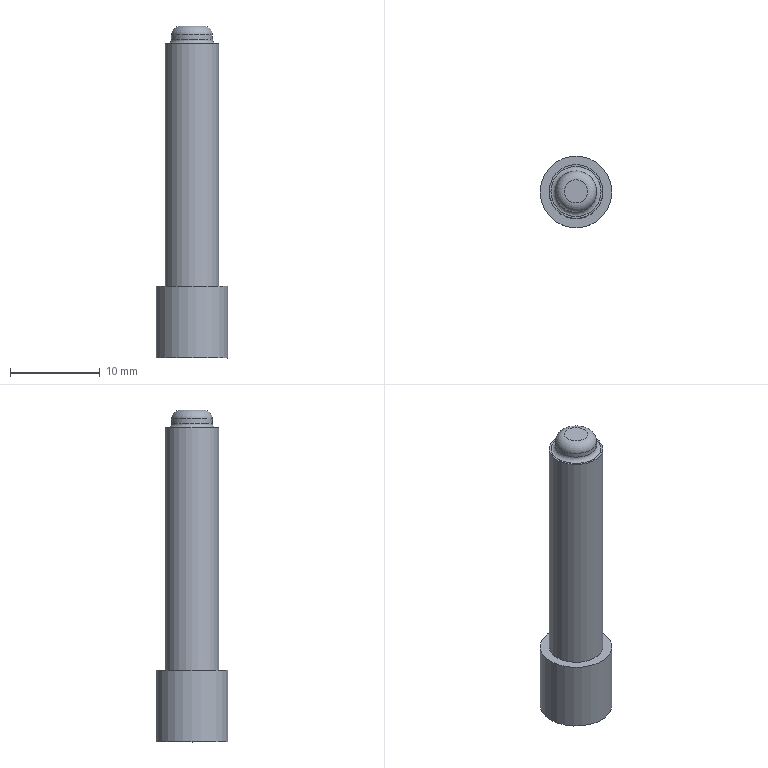Part | NX | features solid 2 | 1 solid | 9 faces | box 8 x 8 x 37 mm | volume 1197 mm3 | plane 4 | cylinder 3 | torus 2 | commonest cylinder face diameters 4.58 x1 6 x1 8 x1
STEP:
#1=CARTESIAN_POINT('',(4220.236,-877.122,858.716));
#2=VERTEX_POINT('',#1);
#3=CARTESIAN_POINT('',(4217.236,-877.122,858.716));
#4=DIRECTION('',(0.,0.,1.));
#5=DIRECTION('',(1.,0.,0.));
#6=AXIS2_PLACEMENT_3D('',#3,#4,#5);
#7=CIRCLE('',#6,3.);
#8=EDGE_CURVE('',#2,#2,#7,.T.);
#9=ORIENTED_EDGE('',*,*,#8,.F.);
#10=EDGE_LOOP('',(#9));
#11=FACE_BOUND('',#10,.T.);
#12=CARTESIAN_POINT('',(4214.236,-877.122,831.716));
#13=VERTEX_POINT('',#12);
#14=CARTESIAN_POINT('',(4217.236,-877.122,831.716));
#15=DIRECTION('',(0.,0.,-1.));
#16=DIRECTION('',(-1.,0.,0.));
#17=AXIS2_PLACEMENT_3D('',#14,#15,#16);
#18=CIRCLE('',#17,3.);
#19=EDGE_CURVE('',#13,#13,#18,.F.);
#20=ORIENTED_EDGE('',*,*,#19,.T.);
#21=EDGE_LOOP('',(#20));
#22=FACE_BOUND('',#21,.T.);
#23=CARTESIAN_POINT('',(4217.236,-877.122,823.716));
#24=DIRECTION('',(0.,0.,1.));
#25=DIRECTION('',(1.,0.,0.));
#26=AXIS2_PLACEMENT_3D('',#23,#24,#25);
#27=CYLINDRICAL_SURFACE('',#26,3.);
#28=ADVANCED_FACE('',(#11,#22),#27,.T.);
#29=CARTESIAN_POINT('',(4214.997,-877.601,859.716));
#30=VERTEX_POINT('',#29);
#31=CARTESIAN_POINT('',(4215.858,-879.254,859.716));
#32=CARTESIAN_POINT('',(4214.754,-877.652,859.716));
#33=CARTESIAN_POINT('',(4215.107,-875.742,859.716));
#34=CARTESIAN_POINT('',(4216.704,-874.641,859.716));
#35=CARTESIAN_POINT('',(4218.615,-874.991,859.716));
#36=CARTESIAN_POINT('',(4219.718,-876.591,859.716));
#37=CARTESIAN_POINT('',(4219.367,-878.499,859.716));
#38=CARTESIAN_POINT('',(4217.769,-879.603,859.716));
#39=CARTESIAN_POINT('',(4215.858,-879.254,859.716));
#40=CARTESIAN_POINT('',(4214.754,-877.652,859.716));
#41=CARTESIAN_POINT('',(4215.107,-875.742,859.716));
#42=B_SPLINE_CURVE_WITH_KNOTS('',3,(#31,#32,#33,#34,#35,#36,#37,#38,#39,#40,#41),.UNSPECIFIED.,.T.,.F.,(1,1,1,1,1,1,1,1,1,1,1,1,1,1,1),(-0.005369,-0.003579,-0.00179,0.,0.00179,0.003579,0.005369,0.007159,0.008948,0.01074,0.01253,0.01432,0.01611,0.0179,0.01969),.UNSPECIFIED.);
#43=EDGE_CURVE('',#30,#30,#42,.T.);
#44=ORIENTED_EDGE('',*,*,#43,.T.);
#45=EDGE_LOOP('',(#44));
#46=FACE_BOUND('',#45,.T.);
#47=CARTESIAN_POINT('',(4219.526,-877.122,859.216));
#48=VERTEX_POINT('',#47);
#49=CARTESIAN_POINT('',(4217.236,-877.122,859.216));
#50=DIRECTION('',(0.,0.,1.));
#51=DIRECTION('',(1.,0.,0.));
#52=AXIS2_PLACEMENT_3D('',#49,#50,#51);
#53=CIRCLE('',#52,2.29);
#54=EDGE_CURVE('',#48,#48,#53,.F.);
#55=ORIENTED_EDGE('',*,*,#54,.F.);
#56=EDGE_LOOP('',(#55));
#57=FACE_BOUND('',#56,.T.);
#58=CARTESIAN_POINT('',(4217.236,-877.122,860.716));
#59=DIRECTION('',(0.,0.,-1.));
#60=DIRECTION('',(-1.,0.,0.));
#61=AXIS2_PLACEMENT_3D('',#58,#59,#60);
#62=CYLINDRICAL_SURFACE('',#61,2.29);
#63=ADVANCED_FACE('',(#46,#57),#62,.T.);
#64=CARTESIAN_POINT('',(4215.946,-877.122,860.716));
#65=VERTEX_POINT('',#64);
#66=CARTESIAN_POINT('',(4217.236,-877.122,860.716));
#67=DIRECTION('',(0.,0.,-1.));
#68=DIRECTION('',(-1.,0.,0.));
#69=AXIS2_PLACEMENT_3D('',#66,#67,#68);
#70=CIRCLE('',#69,1.29);
#71=EDGE_CURVE('',#65,#65,#70,.F.);
#72=ORIENTED_EDGE('',*,*,#71,.T.);
#73=EDGE_LOOP('',(#72));
#74=FACE_BOUND('',#73,.T.);
#75=CARTESIAN_POINT('',(4217.236,-877.122,860.716));
#76=DIRECTION('',(0.,0.,-1.));
#77=DIRECTION('',(-1.,0.,0.));
#78=AXIS2_PLACEMENT_3D('',#75,#76,#77);
#79=PLANE('',#78);
#80=ADVANCED_FACE('',(#74),#79,.F.);
#81=CARTESIAN_POINT('',(4220.026,-877.122,858.716));
#82=VERTEX_POINT('',#81);
#83=CARTESIAN_POINT('',(4217.236,-877.122,858.716));
#84=DIRECTION('',(0.,0.,1.));
#85=DIRECTION('',(1.,0.,0.));
#86=AXIS2_PLACEMENT_3D('',#83,#84,#85);
#87=CIRCLE('',#86,2.79);
#88=EDGE_CURVE('',#82,#82,#87,.F.);
#89=ORIENTED_EDGE('',*,*,#88,.F.);
#90=EDGE_LOOP('',(#89));
#91=FACE_BOUND('',#90,.T.);
#92=ORIENTED_EDGE('',*,*,#54,.T.);
#93=EDGE_LOOP('',(#92));
#94=FACE_BOUND('',#93,.T.);
#95=CARTESIAN_POINT('',(4217.236,-877.122,859.216));
#96=DIRECTION('',(0.,0.,1.));
#97=DIRECTION('',(1.,0.,0.));
#98=AXIS2_PLACEMENT_3D('',#95,#96,#97);
#99=TOROIDAL_SURFACE('',#98,2.79,0.5);
#100=ADVANCED_FACE('',(#91,#94),#99,.F.);
#101=ORIENTED_EDGE('',*,*,#88,.T.);
#102=EDGE_LOOP('',(#101));
#103=FACE_BOUND('',#102,.T.);
#104=ORIENTED_EDGE('',*,*,#8,.T.);
#105=EDGE_LOOP('',(#104));
#106=FACE_BOUND('',#105,.T.);
#107=CARTESIAN_POINT('',(4217.236,-839.122,858.716));
#108=DIRECTION('',(0.,0.,1.));
#109=DIRECTION('',(1.,0.,0.));
#110=AXIS2_PLACEMENT_3D('',#107,#108,#109);
#111=PLANE('',#110);
#112=ADVANCED_FACE('',(#103,#106),#111,.T.);
#113=ORIENTED_EDGE('',*,*,#71,.F.);
#114=EDGE_LOOP('',(#113));
#115=FACE_BOUND('',#114,.T.);
#116=ORIENTED_EDGE('',*,*,#43,.F.);
#117=EDGE_LOOP('',(#116));
#118=FACE_BOUND('',#117,.T.);
#119=CARTESIAN_POINT('',(4217.236,-877.122,859.716));
#120=DIRECTION('',(0.,0.,-1.));
#121=DIRECTION('',(-1.,0.,0.));
#122=AXIS2_PLACEMENT_3D('',#119,#120,#121);
#123=TOROIDAL_SURFACE('',#122,1.29,1.);
#124=ADVANCED_FACE('',(#115,#118),#123,.T.);
#125=CARTESIAN_POINT('',(4213.236,-877.122,823.716));
#126=VERTEX_POINT('',#125);
#127=CARTESIAN_POINT('',(4217.236,-877.122,823.716));
#128=DIRECTION('',(0.,0.,-1.));
#129=DIRECTION('',(-1.,0.,0.));
#130=AXIS2_PLACEMENT_3D('',#127,#128,#129);
#131=CIRCLE('',#130,4.);
#132=EDGE_CURVE('',#126,#126,#131,.T.);
#133=ORIENTED_EDGE('',*,*,#132,.T.);
#134=EDGE_LOOP('',(#133));
#135=FACE_BOUND('',#134,.T.);
#136=CARTESIAN_POINT('',(4217.236,-877.122,823.716));
#137=DIRECTION('',(0.,0.,-1.));
#138=DIRECTION('',(-1.,0.,0.));
#139=AXIS2_PLACEMENT_3D('',#136,#137,#138);
#140=PLANE('',#139);
#141=ADVANCED_FACE('',(#135),#140,.T.);
#142=CARTESIAN_POINT('',(4213.236,-877.122,831.716));
#143=VERTEX_POINT('',#142);
#144=CARTESIAN_POINT('',(4217.236,-877.122,831.716));
#145=DIRECTION('',(0.,0.,-1.));
#146=DIRECTION('',(-1.,0.,0.));
#147=AXIS2_PLACEMENT_3D('',#144,#145,#146);
#148=CIRCLE('',#147,4.);
#149=EDGE_CURVE('',#143,#143,#148,.T.);
#150=ORIENTED_EDGE('',*,*,#149,.T.);
#151=EDGE_LOOP('',(#150));
#152=FACE_BOUND('',#151,.T.);
#153=ORIENTED_EDGE('',*,*,#132,.F.);
#154=EDGE_LOOP('',(#153));
#155=FACE_BOUND('',#154,.T.);
#156=CARTESIAN_POINT('',(4217.236,-877.122,823.716));
#157=DIRECTION('',(0.,0.,1.));
#158=DIRECTION('',(1.,0.,0.));
#159=AXIS2_PLACEMENT_3D('',#156,#157,#158);
#160=CYLINDRICAL_SURFACE('',#159,4.);
#161=ADVANCED_FACE('',(#152,#155),#160,.T.);
#162=ORIENTED_EDGE('',*,*,#19,.F.);
#163=EDGE_LOOP('',(#162));
#164=FACE_BOUND('',#163,.T.);
#165=ORIENTED_EDGE('',*,*,#149,.F.);
#166=EDGE_LOOP('',(#165));
#167=FACE_BOUND('',#166,.T.);
#168=CARTESIAN_POINT('',(4217.236,-877.122,831.716));
#169=DIRECTION('',(0.,0.,-1.));
#170=DIRECTION('',(-1.,0.,0.));
#171=AXIS2_PLACEMENT_3D('',#168,#169,#170);
#172=PLANE('',#171);
#173=ADVANCED_FACE('',(#164,#167),#172,.F.);
#174=CLOSED_SHELL('',(#28,#63,#80,#100,#112,#124,#141,#161,#173));
#175=MANIFOLD_SOLID_BREP('',#174);
#176=(LENGTH_UNIT()NAMED_UNIT(*)SI_UNIT(.MILLI.,.METRE.));
#177=UNCERTAINTY_MEASURE_WITH_UNIT(LENGTH_MEASURE(0.0508),#176,'','');
#178=(NAMED_UNIT(*)PLANE_ANGLE_UNIT()SI_UNIT($,.RADIAN.));
#179=(NAMED_UNIT(*)SI_UNIT($,.STERADIAN.)SOLID_ANGLE_UNIT());
#180=(GEOMETRIC_REPRESENTATION_CONTEXT(3)GLOBAL_UNCERTAINTY_ASSIGNED_CONTEXT((#177))GLOBAL_UNIT_ASSIGNED_CONTEXT((#176,#178,#179))REPRESENTATION_CONTEXT('',''));
#181=ADVANCED_BREP_SHAPE_REPRESENTATION('',(#175),#180);